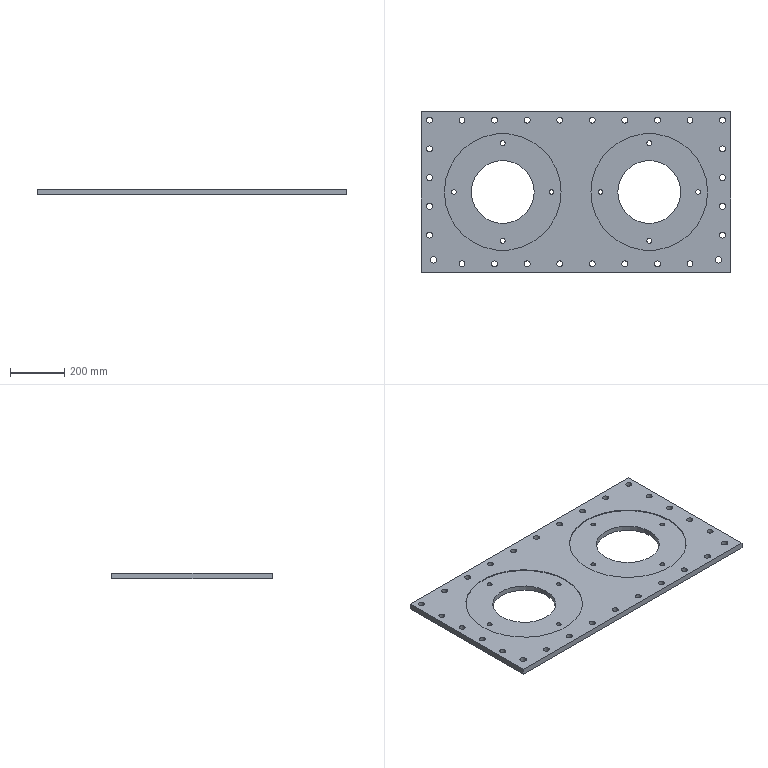Part | SolidWorks | features ICE 3, CirPattern 2, HoleWzd 2, RefAxis 2, Extrusion 1 | 1 solid | 88 faces | box 1140 x 590 x 22 mm | volume 12045594 mm3 | cylinder 80 | plane 8 | commonest cylinder face diameters 22 x52 17.5 x16 24 x4 232 x4 430 x4